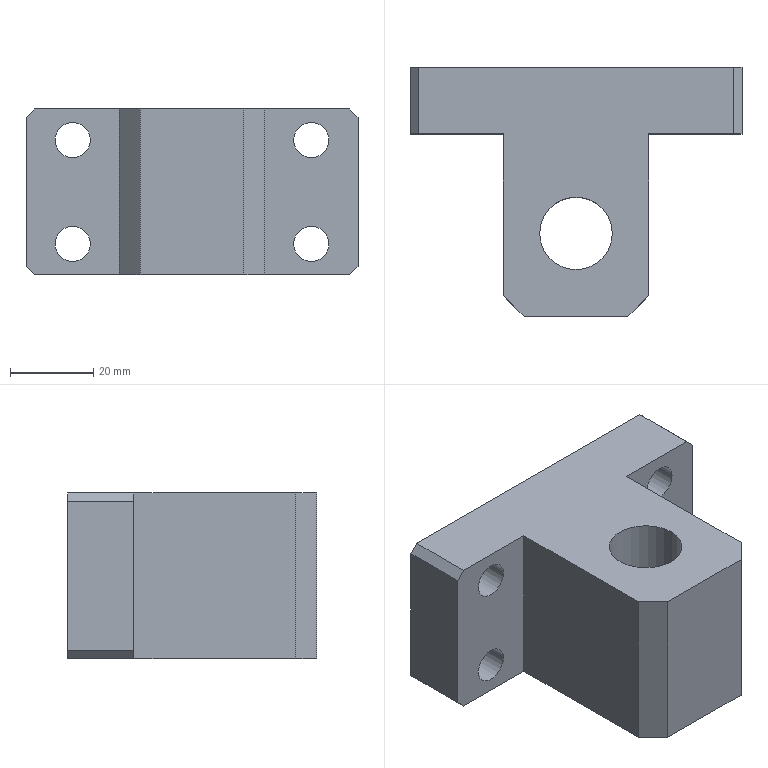Part | STEP file | fBY02F02M-00-26A | 1 solid | 26 faces | box 80 x 60 x 40 mm | volume 98419 mm3 | plane 16 | cylinder 10 | commonest cylinder face diameters 8.5 x8 17.5 x2